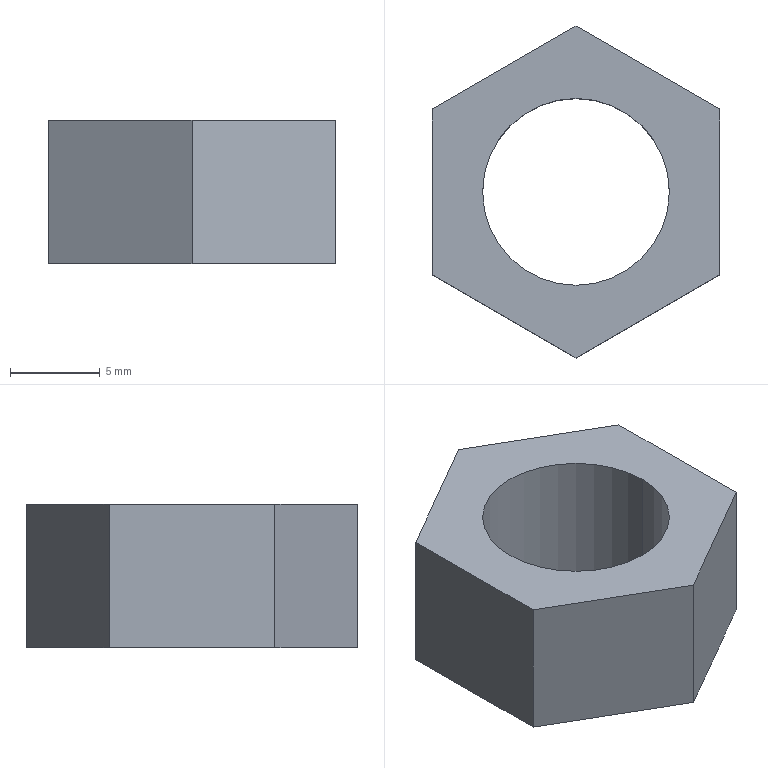Part | SolidWorks | features Extrusion 1 | 1 solid | 10 faces | box 16 x 18.475 x 8 mm | volume 1094 mm3 | plane 8 | cylinder 2 | commonest cylinder face diameters 10.4 x2
STEP:
#1=CARTESIAN_POINT('',(-5.2,0.,8.));
#2=VERTEX_POINT('',#1);
#3=CARTESIAN_POINT('',(5.2,0.,8.));
#4=VERTEX_POINT('',#3);
#5=CARTESIAN_POINT('',(0.,0.,8.));
#6=DIRECTION('',(0.,0.,1.));
#7=DIRECTION('',(1.,0.,0.));
#8=AXIS2_PLACEMENT_3D('',#5,#6,#7);
#9=CIRCLE('',#8,5.2);
#10=EDGE_CURVE('',#2,#4,#9,.T.);
#11=ORIENTED_EDGE('',*,*,#10,.T.);
#12=CARTESIAN_POINT('',(5.2,0.,0.));
#13=VERTEX_POINT('',#12);
#14=CARTESIAN_POINT('',(5.2,0.,8.));
#15=DIRECTION('',(0.,0.,-1.));
#16=VECTOR('',#15,1000.);
#17=LINE('',#14,#16);
#18=EDGE_CURVE('',#4,#13,#17,.T.);
#19=ORIENTED_EDGE('',*,*,#18,.T.);
#20=CARTESIAN_POINT('',(-5.2,0.,0.));
#21=VERTEX_POINT('',#20);
#22=CARTESIAN_POINT('',(0.,0.,0.));
#23=DIRECTION('',(0.,0.,1.));
#24=DIRECTION('',(1.,0.,0.));
#25=AXIS2_PLACEMENT_3D('',#22,#23,#24);
#26=CIRCLE('',#25,5.2);
#27=EDGE_CURVE('',#21,#13,#26,.T.);
#28=ORIENTED_EDGE('',*,*,#27,.F.);
#29=CARTESIAN_POINT('',(-5.2,0.,8.));
#30=DIRECTION('',(0.,0.,-1.));
#31=VECTOR('',#30,1000.);
#32=LINE('',#29,#31);
#33=EDGE_CURVE('',#2,#21,#32,.T.);
#34=ORIENTED_EDGE('',*,*,#33,.F.);
#35=EDGE_LOOP('',(#11,#19,#28,#34));
#36=FACE_OUTER_BOUND('',#35,.T.);
#37=CARTESIAN_POINT('',(0.,0.,8.));
#38=DIRECTION('',(0.,0.,-1.));
#39=DIRECTION('',(-1.,0.,0.));
#40=AXIS2_PLACEMENT_3D('',#37,#38,#39);
#41=CYLINDRICAL_SURFACE('',#40,5.2);
#42=ADVANCED_FACE('',(#36),#41,.F.);
#43=CARTESIAN_POINT('',(8.,4.619,8.));
#44=VERTEX_POINT('',#43);
#45=CARTESIAN_POINT('',(0.,9.238,8.));
#46=VERTEX_POINT('',#45);
#47=CARTESIAN_POINT('',(8.,4.619,8.));
#48=DIRECTION('',(-0.866,0.5,0.));
#49=VECTOR('',#48,1000.);
#50=LINE('',#47,#49);
#51=EDGE_CURVE('',#44,#46,#50,.T.);
#52=ORIENTED_EDGE('',*,*,#51,.T.);
#53=CARTESIAN_POINT('',(-8.,4.619,8.));
#54=VERTEX_POINT('',#53);
#55=CARTESIAN_POINT('',(0.,9.238,8.));
#56=DIRECTION('',(-0.866,-0.5,0.));
#57=VECTOR('',#56,1000.);
#58=LINE('',#55,#57);
#59=EDGE_CURVE('',#46,#54,#58,.T.);
#60=ORIENTED_EDGE('',*,*,#59,.T.);
#61=CARTESIAN_POINT('',(-8.,-4.619,8.));
#62=VERTEX_POINT('',#61);
#63=CARTESIAN_POINT('',(-8.,4.619,8.));
#64=DIRECTION('',(0.,-1.,0.));
#65=VECTOR('',#64,1000.);
#66=LINE('',#63,#65);
#67=EDGE_CURVE('',#54,#62,#66,.T.);
#68=ORIENTED_EDGE('',*,*,#67,.T.);
#69=CARTESIAN_POINT('',(0.,-9.238,8.));
#70=VERTEX_POINT('',#69);
#71=CARTESIAN_POINT('',(-8.,-4.619,8.));
#72=DIRECTION('',(0.866,-0.5,0.));
#73=VECTOR('',#72,1000.);
#74=LINE('',#71,#73);
#75=EDGE_CURVE('',#62,#70,#74,.T.);
#76=ORIENTED_EDGE('',*,*,#75,.T.);
#77=CARTESIAN_POINT('',(8.,-4.619,8.));
#78=VERTEX_POINT('',#77);
#79=CARTESIAN_POINT('',(0.,-9.238,8.));
#80=DIRECTION('',(0.866,0.5,0.));
#81=VECTOR('',#80,1000.);
#82=LINE('',#79,#81);
#83=EDGE_CURVE('',#70,#78,#82,.T.);
#84=ORIENTED_EDGE('',*,*,#83,.T.);
#85=CARTESIAN_POINT('',(8.,-4.619,8.));
#86=DIRECTION('',(0.,1.,0.));
#87=VECTOR('',#86,1000.);
#88=LINE('',#85,#87);
#89=EDGE_CURVE('',#78,#44,#88,.T.);
#90=ORIENTED_EDGE('',*,*,#89,.T.);
#91=EDGE_LOOP('',(#52,#60,#68,#76,#84,#90));
#92=FACE_OUTER_BOUND('',#91,.T.);
#93=ORIENTED_EDGE('',*,*,#10,.F.);
#94=CARTESIAN_POINT('',(0.,0.,8.));
#95=DIRECTION('',(0.,0.,1.));
#96=DIRECTION('',(1.,0.,0.));
#97=AXIS2_PLACEMENT_3D('',#94,#95,#96);
#98=CIRCLE('',#97,5.2);
#99=EDGE_CURVE('',#4,#2,#98,.T.);
#100=ORIENTED_EDGE('',*,*,#99,.F.);
#101=EDGE_LOOP('',(#93,#100));
#102=FACE_BOUND('',#101,.T.);
#103=CARTESIAN_POINT('',(0.,0.,8.));
#104=DIRECTION('',(0.,0.,1.));
#105=DIRECTION('',(1.,0.,0.));
#106=AXIS2_PLACEMENT_3D('',#103,#104,#105);
#107=PLANE('',#106);
#108=ADVANCED_FACE('',(#92,#102),#107,.T.);
#109=CARTESIAN_POINT('',(8.,4.619,0.));
#110=VERTEX_POINT('',#109);
#111=CARTESIAN_POINT('',(0.,9.238,0.));
#112=VERTEX_POINT('',#111);
#113=CARTESIAN_POINT('',(8.,4.619,0.));
#114=DIRECTION('',(-0.866,0.5,0.));
#115=VECTOR('',#114,1000.);
#116=LINE('',#113,#115);
#117=EDGE_CURVE('',#110,#112,#116,.T.);
#118=ORIENTED_EDGE('',*,*,#117,.F.);
#119=CARTESIAN_POINT('',(8.,-4.619,0.));
#120=VERTEX_POINT('',#119);
#121=CARTESIAN_POINT('',(8.,-4.619,0.));
#122=DIRECTION('',(0.,1.,0.));
#123=VECTOR('',#122,1000.);
#124=LINE('',#121,#123);
#125=EDGE_CURVE('',#120,#110,#124,.T.);
#126=ORIENTED_EDGE('',*,*,#125,.F.);
#127=CARTESIAN_POINT('',(0.,-9.238,0.));
#128=VERTEX_POINT('',#127);
#129=CARTESIAN_POINT('',(0.,-9.238,0.));
#130=DIRECTION('',(0.866,0.5,0.));
#131=VECTOR('',#130,1000.);
#132=LINE('',#129,#131);
#133=EDGE_CURVE('',#128,#120,#132,.T.);
#134=ORIENTED_EDGE('',*,*,#133,.F.);
#135=CARTESIAN_POINT('',(-8.,-4.619,0.));
#136=VERTEX_POINT('',#135);
#137=CARTESIAN_POINT('',(-8.,-4.619,0.));
#138=DIRECTION('',(0.866,-0.5,0.));
#139=VECTOR('',#138,1000.);
#140=LINE('',#137,#139);
#141=EDGE_CURVE('',#136,#128,#140,.T.);
#142=ORIENTED_EDGE('',*,*,#141,.F.);
#143=CARTESIAN_POINT('',(-8.,4.619,0.));
#144=VERTEX_POINT('',#143);
#145=CARTESIAN_POINT('',(-8.,4.619,0.));
#146=DIRECTION('',(0.,-1.,0.));
#147=VECTOR('',#146,1000.);
#148=LINE('',#145,#147);
#149=EDGE_CURVE('',#144,#136,#148,.T.);
#150=ORIENTED_EDGE('',*,*,#149,.F.);
#151=CARTESIAN_POINT('',(0.,9.238,0.));
#152=DIRECTION('',(-0.866,-0.5,0.));
#153=VECTOR('',#152,1000.);
#154=LINE('',#151,#153);
#155=EDGE_CURVE('',#112,#144,#154,.T.);
#156=ORIENTED_EDGE('',*,*,#155,.F.);
#157=EDGE_LOOP('',(#118,#126,#134,#142,#150,#156));
#158=FACE_OUTER_BOUND('',#157,.T.);
#159=ORIENTED_EDGE('',*,*,#27,.T.);
#160=CARTESIAN_POINT('',(0.,0.,0.));
#161=DIRECTION('',(0.,0.,1.));
#162=DIRECTION('',(1.,0.,0.));
#163=AXIS2_PLACEMENT_3D('',#160,#161,#162);
#164=CIRCLE('',#163,5.2);
#165=EDGE_CURVE('',#13,#21,#164,.T.);
#166=ORIENTED_EDGE('',*,*,#165,.T.);
#167=EDGE_LOOP('',(#159,#166));
#168=FACE_BOUND('',#167,.T.);
#169=CARTESIAN_POINT('',(0.,0.,0.));
#170=DIRECTION('',(0.,0.,1.));
#171=DIRECTION('',(1.,0.,0.));
#172=AXIS2_PLACEMENT_3D('',#169,#170,#171);
#173=PLANE('',#172);
#174=ADVANCED_FACE('',(#158,#168),#173,.F.);
#175=ORIENTED_EDGE('',*,*,#117,.T.);
#176=CARTESIAN_POINT('',(0.,9.238,8.));
#177=DIRECTION('',(0.,0.,-1.));
#178=VECTOR('',#177,1000.);
#179=LINE('',#176,#178);
#180=EDGE_CURVE('',#46,#112,#179,.T.);
#181=ORIENTED_EDGE('',*,*,#180,.F.);
#182=ORIENTED_EDGE('',*,*,#51,.F.);
#183=CARTESIAN_POINT('',(8.,4.619,8.));
#184=DIRECTION('',(0.,0.,-1.));
#185=VECTOR('',#184,1000.);
#186=LINE('',#183,#185);
#187=EDGE_CURVE('',#44,#110,#186,.T.);
#188=ORIENTED_EDGE('',*,*,#187,.T.);
#189=EDGE_LOOP('',(#175,#181,#182,#188));
#190=FACE_OUTER_BOUND('',#189,.T.);
#191=CARTESIAN_POINT('',(8.,4.619,8.));
#192=DIRECTION('',(-0.5,-0.866,0.));
#193=DIRECTION('',(0.866,-0.5,0.));
#194=AXIS2_PLACEMENT_3D('',#191,#192,#193);
#195=PLANE('',#194);
#196=ADVANCED_FACE('',(#190),#195,.F.);
#197=ORIENTED_EDGE('',*,*,#155,.T.);
#198=CARTESIAN_POINT('',(-8.,4.619,8.));
#199=DIRECTION('',(0.,0.,-1.));
#200=VECTOR('',#199,1000.);
#201=LINE('',#198,#200);
#202=EDGE_CURVE('',#54,#144,#201,.T.);
#203=ORIENTED_EDGE('',*,*,#202,.F.);
#204=ORIENTED_EDGE('',*,*,#59,.F.);
#205=ORIENTED_EDGE('',*,*,#180,.T.);
#206=EDGE_LOOP('',(#197,#203,#204,#205));
#207=FACE_OUTER_BOUND('',#206,.T.);
#208=CARTESIAN_POINT('',(0.,9.238,8.));
#209=DIRECTION('',(0.5,-0.866,0.));
#210=DIRECTION('',(0.866,0.5,0.));
#211=AXIS2_PLACEMENT_3D('',#208,#209,#210);
#212=PLANE('',#211);
#213=ADVANCED_FACE('',(#207),#212,.F.);
#214=ORIENTED_EDGE('',*,*,#149,.T.);
#215=CARTESIAN_POINT('',(-8.,-4.619,8.));
#216=DIRECTION('',(0.,0.,-1.));
#217=VECTOR('',#216,1000.);
#218=LINE('',#215,#217);
#219=EDGE_CURVE('',#62,#136,#218,.T.);
#220=ORIENTED_EDGE('',*,*,#219,.F.);
#221=ORIENTED_EDGE('',*,*,#67,.F.);
#222=ORIENTED_EDGE('',*,*,#202,.T.);
#223=EDGE_LOOP('',(#214,#220,#221,#222));
#224=FACE_OUTER_BOUND('',#223,.T.);
#225=CARTESIAN_POINT('',(-8.,4.619,8.));
#226=DIRECTION('',(1.,0.,0.));
#227=DIRECTION('',(0.,1.,0.));
#228=AXIS2_PLACEMENT_3D('',#225,#226,#227);
#229=PLANE('',#228);
#230=ADVANCED_FACE('',(#224),#229,.F.);
#231=ORIENTED_EDGE('',*,*,#141,.T.);
#232=CARTESIAN_POINT('',(0.,-9.238,8.));
#233=DIRECTION('',(0.,0.,-1.));
#234=VECTOR('',#233,1000.);
#235=LINE('',#232,#234);
#236=EDGE_CURVE('',#70,#128,#235,.T.);
#237=ORIENTED_EDGE('',*,*,#236,.F.);
#238=ORIENTED_EDGE('',*,*,#75,.F.);
#239=ORIENTED_EDGE('',*,*,#219,.T.);
#240=EDGE_LOOP('',(#231,#237,#238,#239));
#241=FACE_OUTER_BOUND('',#240,.T.);
#242=CARTESIAN_POINT('',(-8.,-4.619,8.));
#243=DIRECTION('',(0.5,0.866,0.));
#244=DIRECTION('',(-0.866,0.5,0.));
#245=AXIS2_PLACEMENT_3D('',#242,#243,#244);
#246=PLANE('',#245);
#247=ADVANCED_FACE('',(#241),#246,.F.);
#248=ORIENTED_EDGE('',*,*,#133,.T.);
#249=CARTESIAN_POINT('',(8.,-4.619,8.));
#250=DIRECTION('',(0.,0.,-1.));
#251=VECTOR('',#250,1000.);
#252=LINE('',#249,#251);
#253=EDGE_CURVE('',#78,#120,#252,.T.);
#254=ORIENTED_EDGE('',*,*,#253,.F.);
#255=ORIENTED_EDGE('',*,*,#83,.F.);
#256=ORIENTED_EDGE('',*,*,#236,.T.);
#257=EDGE_LOOP('',(#248,#254,#255,#256));
#258=FACE_OUTER_BOUND('',#257,.T.);
#259=CARTESIAN_POINT('',(0.,-9.238,8.));
#260=DIRECTION('',(-0.5,0.866,0.));
#261=DIRECTION('',(-0.866,-0.5,0.));
#262=AXIS2_PLACEMENT_3D('',#259,#260,#261);
#263=PLANE('',#262);
#264=ADVANCED_FACE('',(#258),#263,.F.);
#265=ORIENTED_EDGE('',*,*,#125,.T.);
#266=ORIENTED_EDGE('',*,*,#187,.F.);
#267=ORIENTED_EDGE('',*,*,#89,.F.);
#268=ORIENTED_EDGE('',*,*,#253,.T.);
#269=EDGE_LOOP('',(#265,#266,#267,#268));
#270=FACE_OUTER_BOUND('',#269,.T.);
#271=CARTESIAN_POINT('',(8.,-4.619,8.));
#272=DIRECTION('',(-1.,0.,0.));
#273=DIRECTION('',(0.,-1.,0.));
#274=AXIS2_PLACEMENT_3D('',#271,#272,#273);
#275=PLANE('',#274);
#276=ADVANCED_FACE('',(#270),#275,.F.);
#277=ORIENTED_EDGE('',*,*,#18,.F.);
#278=ORIENTED_EDGE('',*,*,#99,.T.);
#279=ORIENTED_EDGE('',*,*,#33,.T.);
#280=ORIENTED_EDGE('',*,*,#165,.F.);
#281=EDGE_LOOP('',(#277,#278,#279,#280));
#282=FACE_OUTER_BOUND('',#281,.T.);
#283=CARTESIAN_POINT('',(0.,0.,8.));
#284=DIRECTION('',(0.,0.,-1.));
#285=DIRECTION('',(-1.,0.,0.));
#286=AXIS2_PLACEMENT_3D('',#283,#284,#285);
#287=CYLINDRICAL_SURFACE('',#286,5.2);
#288=ADVANCED_FACE('',(#282),#287,.F.);
#289=CLOSED_SHELL('',(#42,#108,#174,#196,#213,#230,#247,#264,#276,#288));
#290=MANIFOLD_SOLID_BREP('',#289);
#291=CARTESIAN_POINT('',(0.,0.,0.));
#292=DIRECTION('',(0.,0.,1.));
#293=DIRECTION('',(1.,0.,0.));
#294=AXIS2_PLACEMENT_3D('',#291,#292,#293);
#295=(LENGTH_UNIT()NAMED_UNIT(*)SI_UNIT(.MILLI.,.METRE.));
#296=UNCERTAINTY_MEASURE_WITH_UNIT(LENGTH_MEASURE(0.00001),#295,'','');
#297=(NAMED_UNIT(*)PLANE_ANGLE_UNIT()SI_UNIT($,.RADIAN.));
#298=(NAMED_UNIT(*)SI_UNIT($,.STERADIAN.)SOLID_ANGLE_UNIT());
#299=(GEOMETRIC_REPRESENTATION_CONTEXT(3)GLOBAL_UNCERTAINTY_ASSIGNED_CONTEXT((#296))GLOBAL_UNIT_ASSIGNED_CONTEXT((#295,#297,#298))REPRESENTATION_CONTEXT('',''));
#300=ADVANCED_BREP_SHAPE_REPRESENTATION('',(#290,#294),#299);